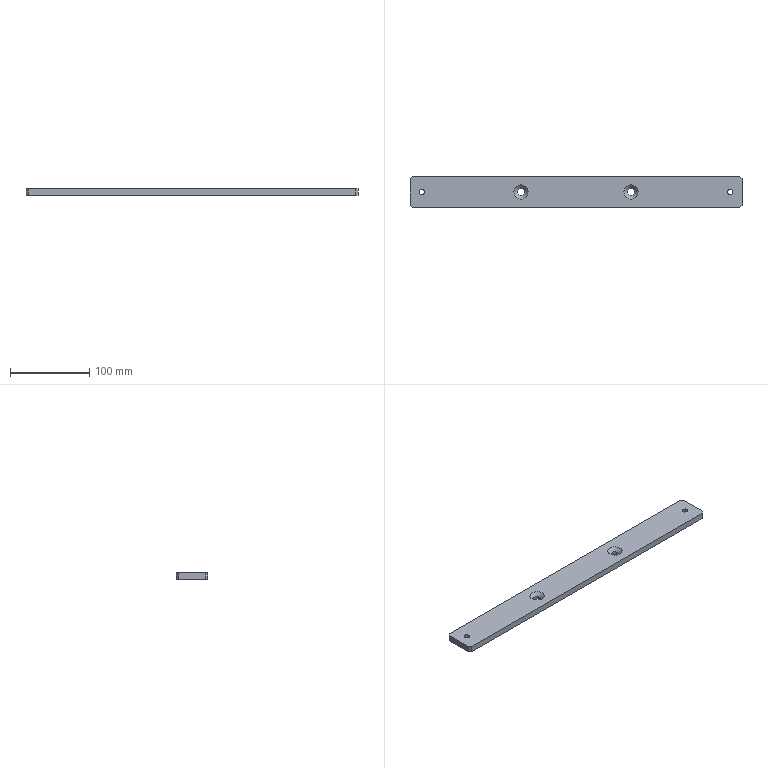Part | STEP file | rectangular profile 40x8-419 | 1 solid | 16 faces | box 418.8 x 40 x 8 mm | volume 131536 mm3 | plane 10 | spline 6